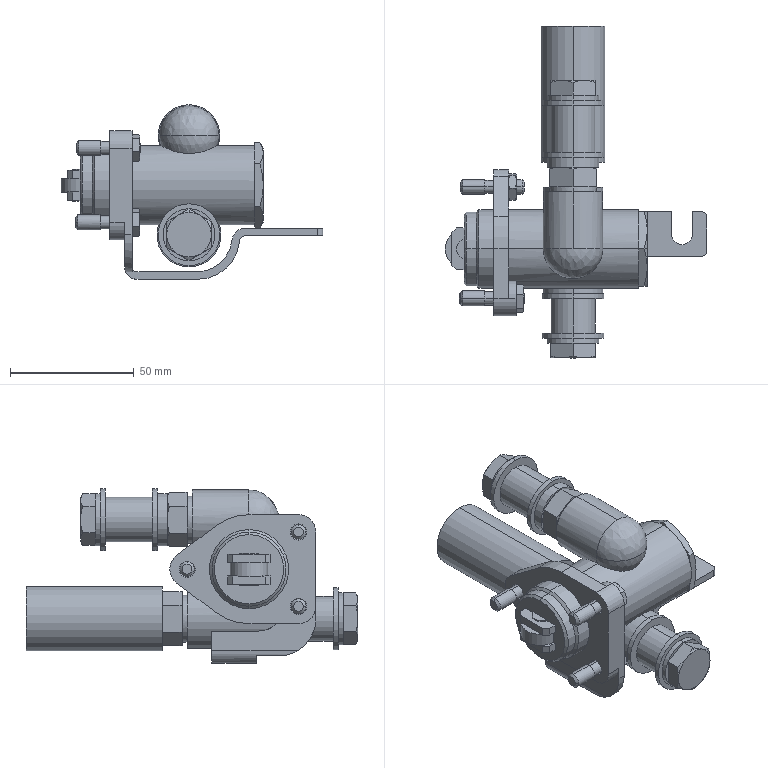Part | SolidWorks | features BaseBody 1 | 1 solid | 341 faces | box 105.638 x 134 x 70.5 mm | volume 159620 mm3 | plane 150 | cone 99 | cylinder 90 | spline 2 | commonest cylinder face diameters 6 x18 25 x8 5.3 x6 6.5 x6 21 x6 4 x4